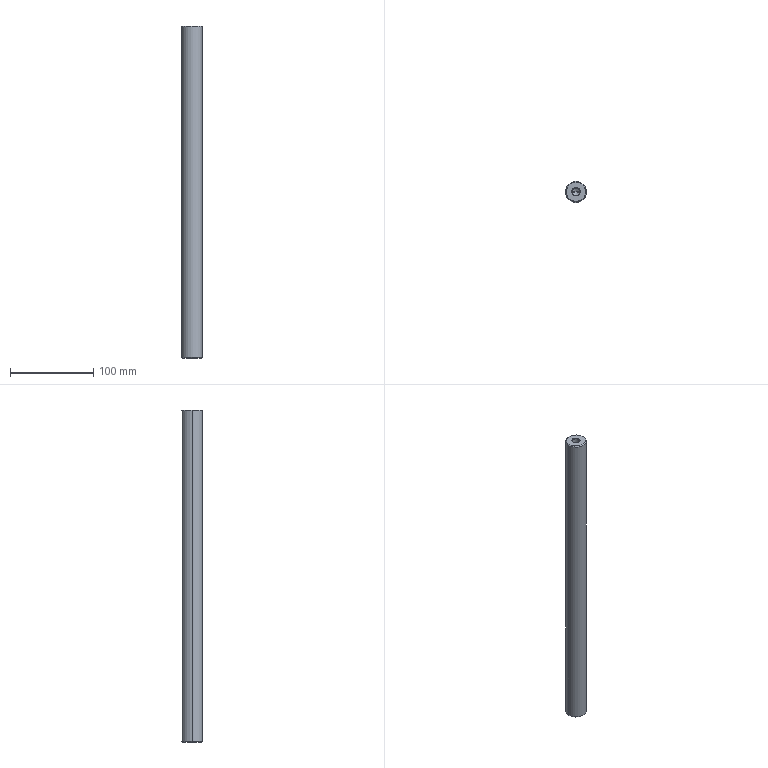Part | STEP file | 1 solid | 20 faces | box 25 x 25 x 400 mm | volume 193039 mm3 | cone 12 | cylinder 6 | plane 2 | commonest cylinder face diameters 8.5 x4 25 x2
STEP:
#1=CARTESIAN_POINT('',(0.,0.,0.));
#2=DIRECTION('',(0.,0.,1.));
#3=DIRECTION('',(1.,0.,0.));
#4=AXIS2_PLACEMENT_3D('',#1,#2,#3);
#5=CARTESIAN_POINT('',(-4.25,0.,-199.225));
#6=VERTEX_POINT('',#5);
#7=CARTESIAN_POINT('',(-5.025,0.,-200.));
#8=VERTEX_POINT('',#7);
#9=CARTESIAN_POINT('',(-5.025,0.,-200.));
#10=DIRECTION('',(-0.7071,0.,-0.7071));
#11=VECTOR('',#10,1.);
#12=LINE('',#9,#11);
#13=CARTESIAN_POINT('',(0.,0.,-200.));
#14=DIRECTION('',(0.,0.,-1.));
#15=DIRECTION('',(-1.,0.,0.));
#16=AXIS2_PLACEMENT_3D('',#13,#14,#15);
#17=CONICAL_SURFACE('',#16,5.025,0.7854);
#18=CARTESIAN_POINT('',(6.283,0.));
#19=DIRECTION('',(0.,1.));
#20=VECTOR('',#19,1.);
#21=LINE('',#18,#20);
#22=(GEOMETRIC_REPRESENTATION_CONTEXT(2)PARAMETRIC_REPRESENTATION_CONTEXT()REPRESENTATION_CONTEXT('',''));
#23=DEFINITIONAL_REPRESENTATION('',(#21),#22);
#24=PCURVE('',#17,#23);
#25=CARTESIAN_POINT('',(0.,0.,-200.));
#26=DIRECTION('',(0.,0.,-1.));
#27=DIRECTION('',(-1.,0.,0.));
#28=AXIS2_PLACEMENT_3D('',#25,#26,#27);
#29=CONICAL_SURFACE('',#28,5.025,0.7854);
#30=CARTESIAN_POINT('',(0.,0.));
#31=DIRECTION('',(0.,1.));
#32=VECTOR('',#31,1.);
#33=LINE('',#30,#32);
#34=(GEOMETRIC_REPRESENTATION_CONTEXT(2)PARAMETRIC_REPRESENTATION_CONTEXT()REPRESENTATION_CONTEXT('',''));
#35=DEFINITIONAL_REPRESENTATION('',(#33),#34);
#36=PCURVE('',#29,#35);
#37=SURFACE_CURVE('',#12,(#24,#36),.PCURVE_S1.);
#38=EDGE_CURVE('',#6,#8,#37,.T.);
#39=ORIENTED_EDGE('',*,*,#38,.T.);
#40=CARTESIAN_POINT('',(5.025,0.,-200.));
#41=VERTEX_POINT('',#40);
#42=CARTESIAN_POINT('',(0.,0.,-200.));
#43=DIRECTION('',(0.,0.,-1.));
#44=DIRECTION('',(-1.,0.,0.));
#45=AXIS2_PLACEMENT_3D('',#42,#43,#44);
#46=CIRCLE('',#45,5.025);
#47=CARTESIAN_POINT('',(0.,0.));
#48=DIRECTION('',(1.,0.));
#49=VECTOR('',#48,1.);
#50=LINE('',#47,#49);
#51=(GEOMETRIC_REPRESENTATION_CONTEXT(2)PARAMETRIC_REPRESENTATION_CONTEXT()REPRESENTATION_CONTEXT('',''));
#52=DEFINITIONAL_REPRESENTATION('',(#50),#51);
#53=PCURVE('',#17,#52);
#54=CARTESIAN_POINT('',(0.,0.,-200.));
#55=DIRECTION('',(0.,0.,1.));
#56=DIRECTION('',(1.,0.,0.));
#57=AXIS2_PLACEMENT_3D('',#54,#55,#56);
#58=PLANE('',#57);
#59=CARTESIAN_POINT('',(-5.025,0.));
#60=CARTESIAN_POINT('',(-5.025,8.704));
#61=CARTESIAN_POINT('',(2.513,4.352));
#62=CARTESIAN_POINT('',(10.05,0.));
#63=CARTESIAN_POINT('',(2.513,-4.352));
#64=CARTESIAN_POINT('',(-5.025,-8.704));
#65=CARTESIAN_POINT('',(-5.025,0.));
#66=(BOUNDED_CURVE()B_SPLINE_CURVE(2,(#59,#60,#61,#62,#63,#64,#65),.UNSPECIFIED.,.T.,.F.)B_SPLINE_CURVE_WITH_KNOTS((1,2,2,2,2,1),(-2.094,0.,2.094,4.189,6.283,8.378),.UNSPECIFIED.)CURVE()GEOMETRIC_REPRESENTATION_ITEM()RATIONAL_B_SPLINE_CURVE((1.,0.5,1.,0.5,1.,0.5,1.))REPRESENTATION_ITEM(''));
#67=(GEOMETRIC_REPRESENTATION_CONTEXT(2)PARAMETRIC_REPRESENTATION_CONTEXT()REPRESENTATION_CONTEXT('',''));
#68=DEFINITIONAL_REPRESENTATION('',(#66),#67);
#69=PCURVE('',#58,#68);
#70=SURFACE_CURVE('',#46,(#53,#69),.PCURVE_S1.);
#71=EDGE_CURVE('',#41,#8,#70,.T.);
#72=ORIENTED_EDGE('',*,*,#71,.F.);
#73=CARTESIAN_POINT('',(4.25,0.,-199.225));
#74=VERTEX_POINT('',#73);
#75=CARTESIAN_POINT('',(5.025,0.,-200.));
#76=DIRECTION('',(0.7071,0.,-0.7071));
#77=VECTOR('',#76,1.);
#78=LINE('',#75,#77);
#79=CARTESIAN_POINT('',(3.142,0.));
#80=DIRECTION('',(0.,1.));
#81=VECTOR('',#80,1.);
#82=LINE('',#79,#81);
#83=(GEOMETRIC_REPRESENTATION_CONTEXT(2)PARAMETRIC_REPRESENTATION_CONTEXT()REPRESENTATION_CONTEXT('',''));
#84=DEFINITIONAL_REPRESENTATION('',(#82),#83);
#85=PCURVE('',#17,#84);
#86=CARTESIAN_POINT('',(3.142,0.));
#87=DIRECTION('',(0.,1.));
#88=VECTOR('',#87,1.);
#89=LINE('',#86,#88);
#90=(GEOMETRIC_REPRESENTATION_CONTEXT(2)PARAMETRIC_REPRESENTATION_CONTEXT()REPRESENTATION_CONTEXT('',''));
#91=DEFINITIONAL_REPRESENTATION('',(#89),#90);
#92=PCURVE('',#29,#91);
#93=SURFACE_CURVE('',#78,(#85,#92),.PCURVE_S1.);
#94=EDGE_CURVE('',#74,#41,#93,.T.);
#95=ORIENTED_EDGE('',*,*,#94,.F.);
#96=CARTESIAN_POINT('',(0.,0.,-199.225));
#97=DIRECTION('',(0.,0.,-1.));
#98=DIRECTION('',(-1.,0.,0.));
#99=AXIS2_PLACEMENT_3D('',#96,#97,#98);
#100=CIRCLE('',#99,4.25);
#101=CARTESIAN_POINT('',(0.,-0.775));
#102=DIRECTION('',(1.,0.));
#103=VECTOR('',#102,1.);
#104=LINE('',#101,#103);
#105=(GEOMETRIC_REPRESENTATION_CONTEXT(2)PARAMETRIC_REPRESENTATION_CONTEXT()REPRESENTATION_CONTEXT('',''));
#106=DEFINITIONAL_REPRESENTATION('',(#104),#105);
#107=PCURVE('',#17,#106);
#108=CARTESIAN_POINT('',(0.,0.,-200.));
#109=DIRECTION('',(0.,0.,-1.));
#110=DIRECTION('',(-1.,0.,0.));
#111=AXIS2_PLACEMENT_3D('',#108,#109,#110);
#112=CYLINDRICAL_SURFACE('',#111,4.25);
#113=CARTESIAN_POINT('',(0.,-0.775));
#114=DIRECTION('',(1.,0.));
#115=VECTOR('',#114,1.);
#116=LINE('',#113,#115);
#117=(GEOMETRIC_REPRESENTATION_CONTEXT(2)PARAMETRIC_REPRESENTATION_CONTEXT()REPRESENTATION_CONTEXT('',''));
#118=DEFINITIONAL_REPRESENTATION('',(#116),#117);
#119=PCURVE('',#112,#118);
#120=SURFACE_CURVE('',#100,(#107,#119),.PCURVE_S1.);
#121=EDGE_CURVE('',#74,#6,#120,.T.);
#122=ORIENTED_EDGE('',*,*,#121,.T.);
#123=EDGE_LOOP('',(#39,#72,#95,#122));
#124=FACE_BOUND('',#123,.F.);
#125=ADVANCED_FACE('',(#124),#17,.F.);
#126=CARTESIAN_POINT('',(-4.25,0.,-172.5));
#127=VERTEX_POINT('',#126);
#128=CARTESIAN_POINT('',(-4.25,0.,-200.));
#129=DIRECTION('',(0.,0.,-1.));
#130=VECTOR('',#129,1.);
#131=LINE('',#128,#130);
#132=CARTESIAN_POINT('',(6.283,0.));
#133=DIRECTION('',(0.,1.));
#134=VECTOR('',#133,1.);
#135=LINE('',#132,#134);
#136=(GEOMETRIC_REPRESENTATION_CONTEXT(2)PARAMETRIC_REPRESENTATION_CONTEXT()REPRESENTATION_CONTEXT('',''));
#137=DEFINITIONAL_REPRESENTATION('',(#135),#136);
#138=PCURVE('',#112,#137);
#139=CARTESIAN_POINT('',(0.,0.,-200.));
#140=DIRECTION('',(0.,0.,-1.));
#141=DIRECTION('',(-1.,0.,0.));
#142=AXIS2_PLACEMENT_3D('',#139,#140,#141);
#143=CYLINDRICAL_SURFACE('',#142,4.25);
#144=CARTESIAN_POINT('',(0.,0.));
#145=DIRECTION('',(0.,1.));
#146=VECTOR('',#145,1.);
#147=LINE('',#144,#146);
#148=(GEOMETRIC_REPRESENTATION_CONTEXT(2)PARAMETRIC_REPRESENTATION_CONTEXT()REPRESENTATION_CONTEXT('',''));
#149=DEFINITIONAL_REPRESENTATION('',(#147),#148);
#150=PCURVE('',#143,#149);
#151=SURFACE_CURVE('',#131,(#138,#150),.PCURVE_S1.);
#152=EDGE_CURVE('',#127,#6,#151,.T.);
#153=ORIENTED_EDGE('',*,*,#152,.T.);
#154=ORIENTED_EDGE('',*,*,#121,.F.);
#155=CARTESIAN_POINT('',(4.25,0.,-172.5));
#156=VERTEX_POINT('',#155);
#157=CARTESIAN_POINT('',(4.25,0.,-200.));
#158=DIRECTION('',(0.,0.,-1.));
#159=VECTOR('',#158,1.);
#160=LINE('',#157,#159);
#161=CARTESIAN_POINT('',(3.142,0.));
#162=DIRECTION('',(0.,1.));
#163=VECTOR('',#162,1.);
#164=LINE('',#161,#163);
#165=(GEOMETRIC_REPRESENTATION_CONTEXT(2)PARAMETRIC_REPRESENTATION_CONTEXT()REPRESENTATION_CONTEXT('',''));
#166=DEFINITIONAL_REPRESENTATION('',(#164),#165);
#167=PCURVE('',#112,#166);
#168=CARTESIAN_POINT('',(3.142,0.));
#169=DIRECTION('',(0.,1.));
#170=VECTOR('',#169,1.);
#171=LINE('',#168,#170);
#172=(GEOMETRIC_REPRESENTATION_CONTEXT(2)PARAMETRIC_REPRESENTATION_CONTEXT()REPRESENTATION_CONTEXT('',''));
#173=DEFINITIONAL_REPRESENTATION('',(#171),#172);
#174=PCURVE('',#143,#173);
#175=SURFACE_CURVE('',#160,(#167,#174),.PCURVE_S1.);
#176=EDGE_CURVE('',#156,#74,#175,.T.);
#177=ORIENTED_EDGE('',*,*,#176,.F.);
#178=CARTESIAN_POINT('',(0.,0.,-172.5));
#179=DIRECTION('',(0.,0.,-1.));
#180=DIRECTION('',(-1.,0.,0.));
#181=AXIS2_PLACEMENT_3D('',#178,#179,#180);
#182=CIRCLE('',#181,4.25);
#183=CARTESIAN_POINT('',(0.,-27.5));
#184=DIRECTION('',(1.,0.));
#185=VECTOR('',#184,1.);
#186=LINE('',#183,#185);
#187=(GEOMETRIC_REPRESENTATION_CONTEXT(2)PARAMETRIC_REPRESENTATION_CONTEXT()REPRESENTATION_CONTEXT('',''));
#188=DEFINITIONAL_REPRESENTATION('',(#186),#187);
#189=PCURVE('',#112,#188);
#190=CARTESIAN_POINT('',(0.,0.,-172.5));
#191=DIRECTION('',(0.,0.,-1.));
#192=DIRECTION('',(-1.,0.,0.));
#193=AXIS2_PLACEMENT_3D('',#190,#191,#192);
#194=CONICAL_SURFACE('',#193,4.25,1.03);
#195=CARTESIAN_POINT('',(0.,0.));
#196=DIRECTION('',(1.,0.));
#197=VECTOR('',#196,1.);
#198=LINE('',#195,#197);
#199=(GEOMETRIC_REPRESENTATION_CONTEXT(2)PARAMETRIC_REPRESENTATION_CONTEXT()REPRESENTATION_CONTEXT('',''));
#200=DEFINITIONAL_REPRESENTATION('',(#198),#199);
#201=PCURVE('',#194,#200);
#202=SURFACE_CURVE('',#182,(#189,#201),.PCURVE_S1.);
#203=EDGE_CURVE('',#156,#127,#202,.T.);
#204=ORIENTED_EDGE('',*,*,#203,.T.);
#205=EDGE_LOOP('',(#153,#154,#177,#204));
#206=FACE_BOUND('',#205,.F.);
#207=ADVANCED_FACE('',(#206),#112,.F.);
#208=ORIENTED_EDGE('',*,*,#203,.F.);
#209=CARTESIAN_POINT('',(0.,0.,-169.946));
#210=VERTEX_POINT('',#209);
#211=CARTESIAN_POINT('',(4.25,0.,-172.5));
#212=DIRECTION('',(0.8572,0.,-0.515));
#213=VECTOR('',#212,1.);
#214=LINE('',#211,#213);
#215=CARTESIAN_POINT('',(3.142,0.));
#216=DIRECTION('',(0.,1.));
#217=VECTOR('',#216,1.);
#218=LINE('',#215,#217);
#219=(GEOMETRIC_REPRESENTATION_CONTEXT(2)PARAMETRIC_REPRESENTATION_CONTEXT()REPRESENTATION_CONTEXT('',''));
#220=DEFINITIONAL_REPRESENTATION('',(#218),#219);
#221=PCURVE('',#194,#220);
#222=CARTESIAN_POINT('',(0.,0.,-172.5));
#223=DIRECTION('',(0.,0.,-1.));
#224=DIRECTION('',(-1.,0.,0.));
#225=AXIS2_PLACEMENT_3D('',#222,#223,#224);
#226=CONICAL_SURFACE('',#225,4.25,1.03);
#227=CARTESIAN_POINT('',(3.142,0.));
#228=DIRECTION('',(0.,1.));
#229=VECTOR('',#228,1.);
#230=LINE('',#227,#229);
#231=(GEOMETRIC_REPRESENTATION_CONTEXT(2)PARAMETRIC_REPRESENTATION_CONTEXT()REPRESENTATION_CONTEXT('',''));
#232=DEFINITIONAL_REPRESENTATION('',(#230),#231);
#233=PCURVE('',#226,#232);
#234=SURFACE_CURVE('',#214,(#221,#233),.PCURVE_S1.);
#235=EDGE_CURVE('',#210,#156,#234,.T.);
#236=ORIENTED_EDGE('',*,*,#235,.F.);
#237=CARTESIAN_POINT('',(-4.25,0.,-172.5));
#238=DIRECTION('',(-0.8572,0.,-0.515));
#239=VECTOR('',#238,1.);
#240=LINE('',#237,#239);
#241=CARTESIAN_POINT('',(6.283,0.));
#242=DIRECTION('',(0.,1.));
#243=VECTOR('',#242,1.);
#244=LINE('',#241,#243);
#245=(GEOMETRIC_REPRESENTATION_CONTEXT(2)PARAMETRIC_REPRESENTATION_CONTEXT()REPRESENTATION_CONTEXT('',''));
#246=DEFINITIONAL_REPRESENTATION('',(#244),#245);
#247=PCURVE('',#194,#246);
#248=CARTESIAN_POINT('',(0.,0.));
#249=DIRECTION('',(0.,1.));
#250=VECTOR('',#249,1.);
#251=LINE('',#248,#250);
#252=(GEOMETRIC_REPRESENTATION_CONTEXT(2)PARAMETRIC_REPRESENTATION_CONTEXT()REPRESENTATION_CONTEXT('',''));
#253=DEFINITIONAL_REPRESENTATION('',(#251),#252);
#254=PCURVE('',#226,#253);
#255=SURFACE_CURVE('',#240,(#247,#254),.PCURVE_S1.);
#256=EDGE_CURVE('',#210,#127,#255,.T.);
#257=ORIENTED_EDGE('',*,*,#256,.T.);
#258=EDGE_LOOP('',(#208,#236,#257));
#259=FACE_BOUND('',#258,.F.);
#260=ADVANCED_FACE('',(#259),#194,.F.);
#261=CARTESIAN_POINT('',(4.25,0.,199.225));
#262=VERTEX_POINT('',#261);
#263=CARTESIAN_POINT('',(5.025,0.,200.));
#264=VERTEX_POINT('',#263);
#265=CARTESIAN_POINT('',(5.025,0.,200.));
#266=DIRECTION('',(0.7071,0.,0.7071));
#267=VECTOR('',#266,1.);
#268=LINE('',#265,#267);
#269=CARTESIAN_POINT('',(0.,0.,200.));
#270=DIRECTION('',(0.,0.,1.));
#271=DIRECTION('',(1.,0.,0.));
#272=AXIS2_PLACEMENT_3D('',#269,#270,#271);
#273=CONICAL_SURFACE('',#272,5.025,0.7854);
#274=CARTESIAN_POINT('',(6.283,0.));
#275=DIRECTION('',(0.,1.));
#276=VECTOR('',#275,1.);
#277=LINE('',#274,#276);
#278=(GEOMETRIC_REPRESENTATION_CONTEXT(2)PARAMETRIC_REPRESENTATION_CONTEXT()REPRESENTATION_CONTEXT('',''));
#279=DEFINITIONAL_REPRESENTATION('',(#277),#278);
#280=PCURVE('',#273,#279);
#281=CARTESIAN_POINT('',(0.,0.,200.));
#282=DIRECTION('',(0.,0.,1.));
#283=DIRECTION('',(1.,0.,0.));
#284=AXIS2_PLACEMENT_3D('',#281,#282,#283);
#285=CONICAL_SURFACE('',#284,5.025,0.7854);
#286=CARTESIAN_POINT('',(0.,0.));
#287=DIRECTION('',(0.,1.));
#288=VECTOR('',#287,1.);
#289=LINE('',#286,#288);
#290=(GEOMETRIC_REPRESENTATION_CONTEXT(2)PARAMETRIC_REPRESENTATION_CONTEXT()REPRESENTATION_CONTEXT('',''));
#291=DEFINITIONAL_REPRESENTATION('',(#289),#290);
#292=PCURVE('',#285,#291);
#293=SURFACE_CURVE('',#268,(#280,#292),.PCURVE_S1.);
#294=EDGE_CURVE('',#262,#264,#293,.T.);
#295=ORIENTED_EDGE('',*,*,#294,.T.);
#296=CARTESIAN_POINT('',(-5.025,0.,200.));
#297=VERTEX_POINT('',#296);
#298=CARTESIAN_POINT('',(0.,0.,200.));
#299=DIRECTION('',(0.,0.,1.));
#300=DIRECTION('',(1.,0.,0.));
#301=AXIS2_PLACEMENT_3D('',#298,#299,#300);
#302=CIRCLE('',#301,5.025);
#303=CARTESIAN_POINT('',(0.,0.));
#304=DIRECTION('',(1.,0.));
#305=VECTOR('',#304,1.);
#306=LINE('',#303,#305);
#307=(GEOMETRIC_REPRESENTATION_CONTEXT(2)PARAMETRIC_REPRESENTATION_CONTEXT()REPRESENTATION_CONTEXT('',''));
#308=DEFINITIONAL_REPRESENTATION('',(#306),#307);
#309=PCURVE('',#273,#308);
#310=CARTESIAN_POINT('',(0.,0.,200.));
#311=DIRECTION('',(0.,0.,1.));
#312=DIRECTION('',(1.,0.,0.));
#313=AXIS2_PLACEMENT_3D('',#310,#311,#312);
#314=PLANE('',#313);
#315=CARTESIAN_POINT('',(0.,0.));
#316=DIRECTION('',(1.,0.));
#317=AXIS2_PLACEMENT_2D('',#315,#316);
#318=CIRCLE('',#317,5.025);
#319=(GEOMETRIC_REPRESENTATION_CONTEXT(2)PARAMETRIC_REPRESENTATION_CONTEXT()REPRESENTATION_CONTEXT('',''));
#320=DEFINITIONAL_REPRESENTATION('',(#318),#319);
#321=PCURVE('',#314,#320);
#322=SURFACE_CURVE('',#302,(#309,#321),.PCURVE_S1.);
#323=EDGE_CURVE('',#297,#264,#322,.T.);
#324=ORIENTED_EDGE('',*,*,#323,.F.);
#325=CARTESIAN_POINT('',(-4.25,0.,199.225));
#326=VERTEX_POINT('',#325);
#327=CARTESIAN_POINT('',(-5.025,0.,200.));
#328=DIRECTION('',(-0.7071,0.,0.7071));
#329=VECTOR('',#328,1.);
#330=LINE('',#327,#329);
#331=CARTESIAN_POINT('',(3.142,0.));
#332=DIRECTION('',(0.,1.));
#333=VECTOR('',#332,1.);
#334=LINE('',#331,#333);
#335=(GEOMETRIC_REPRESENTATION_CONTEXT(2)PARAMETRIC_REPRESENTATION_CONTEXT()REPRESENTATION_CONTEXT('',''));
#336=DEFINITIONAL_REPRESENTATION('',(#334),#335);
#337=PCURVE('',#273,#336);
#338=CARTESIAN_POINT('',(3.142,0.));
#339=DIRECTION('',(0.,1.));
#340=VECTOR('',#339,1.);
#341=LINE('',#338,#340);
#342=(GEOMETRIC_REPRESENTATION_CONTEXT(2)PARAMETRIC_REPRESENTATION_CONTEXT()REPRESENTATION_CONTEXT('',''));
#343=DEFINITIONAL_REPRESENTATION('',(#341),#342);
#344=PCURVE('',#285,#343);
#345=SURFACE_CURVE('',#330,(#337,#344),.PCURVE_S1.);
#346=EDGE_CURVE('',#326,#297,#345,.T.);
#347=ORIENTED_EDGE('',*,*,#346,.F.);
#348=CARTESIAN_POINT('',(0.,0.,199.225));
#349=DIRECTION('',(0.,0.,1.));
#350=DIRECTION('',(1.,0.,0.));
#351=AXIS2_PLACEMENT_3D('',#348,#349,#350);
#352=CIRCLE('',#351,4.25);
#353=CARTESIAN_POINT('',(0.,-0.775));
#354=DIRECTION('',(1.,0.));
#355=VECTOR('',#354,1.);
#356=LINE('',#353,#355);
#357=(GEOMETRIC_REPRESENTATION_CONTEXT(2)PARAMETRIC_REPRESENTATION_CONTEXT()REPRESENTATION_CONTEXT('',''));
#358=DEFINITIONAL_REPRESENTATION('',(#356),#357);
#359=PCURVE('',#273,#358);
#360=CARTESIAN_POINT('',(0.,0.,200.));
#361=DIRECTION('',(0.,0.,1.));
#362=DIRECTION('',(1.,0.,0.));
#363=AXIS2_PLACEMENT_3D('',#360,#361,#362);
#364=CYLINDRICAL_SURFACE('',#363,4.25);
#365=CARTESIAN_POINT('',(0.,-0.775));
#366=DIRECTION('',(1.,0.));
#367=VECTOR('',#366,1.);
#368=LINE('',#365,#367);
#369=(GEOMETRIC_REPRESENTATION_CONTEXT(2)PARAMETRIC_REPRESENTATION_CONTEXT()REPRESENTATION_CONTEXT('',''));
#370=DEFINITIONAL_REPRESENTATION('',(#368),#369);
#371=PCURVE('',#364,#370);
#372=SURFACE_CURVE('',#352,(#359,#371),.PCURVE_S1.);
#373=EDGE_CURVE('',#326,#262,#372,.T.);
#374=ORIENTED_EDGE('',*,*,#373,.T.);
#375=EDGE_LOOP('',(#295,#324,#347,#374));
#376=FACE_BOUND('',#375,.F.);
#377=ADVANCED_FACE('',(#376),#273,.F.);
#378=CARTESIAN_POINT('',(4.25,0.,172.5));
#379=VERTEX_POINT('',#378);
#380=CARTESIAN_POINT('',(4.25,0.,200.));
#381=DIRECTION('',(0.,0.,1.));
#382=VECTOR('',#381,1.);
#383=LINE('',#380,#382);
#384=CARTESIAN_POINT('',(6.283,0.));
#385=DIRECTION('',(0.,1.));
#386=VECTOR('',#385,1.);
#387=LINE('',#384,#386);
#388=(GEOMETRIC_REPRESENTATION_CONTEXT(2)PARAMETRIC_REPRESENTATION_CONTEXT()REPRESENTATION_CONTEXT('',''));
#389=DEFINITIONAL_REPRESENTATION('',(#387),#388);
#390=PCURVE('',#364,#389);
#391=CARTESIAN_POINT('',(0.,0.,200.));
#392=DIRECTION('',(0.,0.,1.));
#393=DIRECTION('',(1.,0.,0.));
#394=AXIS2_PLACEMENT_3D('',#391,#392,#393);
#395=CYLINDRICAL_SURFACE('',#394,4.25);
#396=CARTESIAN_POINT('',(0.,0.));
#397=DIRECTION('',(0.,1.));
#398=VECTOR('',#397,1.);
#399=LINE('',#396,#398);
#400=(GEOMETRIC_REPRESENTATION_CONTEXT(2)PARAMETRIC_REPRESENTATION_CONTEXT()REPRESENTATION_CONTEXT('',''));
#401=DEFINITIONAL_REPRESENTATION('',(#399),#400);
#402=PCURVE('',#395,#401);
#403=SURFACE_CURVE('',#383,(#390,#402),.PCURVE_S1.);
#404=EDGE_CURVE('',#379,#262,#403,.T.);
#405=ORIENTED_EDGE('',*,*,#404,.T.);
#406=ORIENTED_EDGE('',*,*,#373,.F.);
#407=CARTESIAN_POINT('',(-4.25,0.,172.5));
#408=VERTEX_POINT('',#407);
#409=CARTESIAN_POINT('',(-4.25,0.,200.));
#410=DIRECTION('',(0.,0.,1.));
#411=VECTOR('',#410,1.);
#412=LINE('',#409,#411);
#413=CARTESIAN_POINT('',(3.142,0.));
#414=DIRECTION('',(0.,1.));
#415=VECTOR('',#414,1.);
#416=LINE('',#413,#415);
#417=(GEOMETRIC_REPRESENTATION_CONTEXT(2)PARAMETRIC_REPRESENTATION_CONTEXT()REPRESENTATION_CONTEXT('',''));
#418=DEFINITIONAL_REPRESENTATION('',(#416),#417);
#419=PCURVE('',#364,#418);
#420=CARTESIAN_POINT('',(3.142,0.));
#421=DIRECTION('',(0.,1.));
#422=VECTOR('',#421,1.);
#423=LINE('',#420,#422);
#424=(GEOMETRIC_REPRESENTATION_CONTEXT(2)PARAMETRIC_REPRESENTATION_CONTEXT()REPRESENTATION_CONTEXT('',''));
#425=DEFINITIONAL_REPRESENTATION('',(#423),#424);
#426=PCURVE('',#395,#425);
#427=SURFACE_CURVE('',#412,(#419,#426),.PCURVE_S1.);
#428=EDGE_CURVE('',#408,#326,#427,.T.);
#429=ORIENTED_EDGE('',*,*,#428,.F.);
#430=CARTESIAN_POINT('',(0.,0.,172.5));
#431=DIRECTION('',(0.,0.,1.));
#432=DIRECTION('',(1.,0.,0.));
#433=AXIS2_PLACEMENT_3D('',#430,#431,#432);
#434=CIRCLE('',#433,4.25);
#435=CARTESIAN_POINT('',(0.,-27.5));
#436=DIRECTION('',(1.,0.));
#437=VECTOR('',#436,1.);
#438=LINE('',#435,#437);
#439=(GEOMETRIC_REPRESENTATION_CONTEXT(2)PARAMETRIC_REPRESENTATION_CONTEXT()REPRESENTATION_CONTEXT('',''));
#440=DEFINITIONAL_REPRESENTATION('',(#438),#439);
#441=PCURVE('',#364,#440);
#442=CARTESIAN_POINT('',(0.,0.,172.5));
#443=DIRECTION('',(0.,0.,1.));
#444=DIRECTION('',(1.,0.,0.));
#445=AXIS2_PLACEMENT_3D('',#442,#443,#444);
#446=CONICAL_SURFACE('',#445,4.25,1.03);
#447=CARTESIAN_POINT('',(0.,0.));
#448=DIRECTION('',(1.,0.));
#449=VECTOR('',#448,1.);
#450=LINE('',#447,#449);
#451=(GEOMETRIC_REPRESENTATION_CONTEXT(2)PARAMETRIC_REPRESENTATION_CONTEXT()REPRESENTATION_CONTEXT('',''));
#452=DEFINITIONAL_REPRESENTATION('',(#450),#451);
#453=PCURVE('',#446,#452);
#454=SURFACE_CURVE('',#434,(#441,#453),.PCURVE_S1.);
#455=EDGE_CURVE('',#408,#379,#454,.T.);
#456=ORIENTED_EDGE('',*,*,#455,.T.);
#457=EDGE_LOOP('',(#405,#406,#429,#456));
#458=FACE_BOUND('',#457,.F.);
#459=ADVANCED_FACE('',(#458),#364,.F.);
#460=ORIENTED_EDGE('',*,*,#455,.F.);
#461=CARTESIAN_POINT('',(0.,0.,169.946));
#462=VERTEX_POINT('',#461);
#463=CARTESIAN_POINT('',(-4.25,0.,172.5));
#464=DIRECTION('',(-0.8572,0.,0.515));
#465=VECTOR('',#464,1.);
#466=LINE('',#463,#465);
#467=CARTESIAN_POINT('',(3.142,0.));
#468=DIRECTION('',(0.,1.));
#469=VECTOR('',#468,1.);
#470=LINE('',#467,#469);
#471=(GEOMETRIC_REPRESENTATION_CONTEXT(2)PARAMETRIC_REPRESENTATION_CONTEXT()REPRESENTATION_CONTEXT('',''));
#472=DEFINITIONAL_REPRESENTATION('',(#470),#471);
#473=PCURVE('',#446,#472);
#474=CARTESIAN_POINT('',(0.,0.,172.5));
#475=DIRECTION('',(0.,0.,1.));
#476=DIRECTION('',(1.,0.,0.));
#477=AXIS2_PLACEMENT_3D('',#474,#475,#476);
#478=CONICAL_SURFACE('',#477,4.25,1.03);
#479=CARTESIAN_POINT('',(3.142,0.));
#480=DIRECTION('',(0.,1.));
#481=VECTOR('',#480,1.);
#482=LINE('',#479,#481);
#483=(GEOMETRIC_REPRESENTATION_CONTEXT(2)PARAMETRIC_REPRESENTATION_CONTEXT()REPRESENTATION_CONTEXT('',''));
#484=DEFINITIONAL_REPRESENTATION('',(#482),#483);
#485=PCURVE('',#478,#484);
#486=SURFACE_CURVE('',#466,(#473,#485),.PCURVE_S1.);
#487=EDGE_CURVE('',#462,#408,#486,.T.);
#488=ORIENTED_EDGE('',*,*,#487,.F.);
#489=CARTESIAN_POINT('',(4.25,0.,172.5));
#490=DIRECTION('',(0.8572,0.,0.515));
#491=VECTOR('',#490,1.);
#492=LINE('',#489,#491);
#493=CARTESIAN_POINT('',(6.283,0.));
#494=DIRECTION('',(0.,1.));
#495=VECTOR('',#494,1.);
#496=LINE('',#493,#495);
#497=(GEOMETRIC_REPRESENTATION_CONTEXT(2)PARAMETRIC_REPRESENTATION_CONTEXT()REPRESENTATION_CONTEXT('',''));
#498=DEFINITIONAL_REPRESENTATION('',(#496),#497);
#499=PCURVE('',#446,#498);
#500=CARTESIAN_POINT('',(0.,0.));
#501=DIRECTION('',(0.,1.));
#502=VECTOR('',#501,1.);
#503=LINE('',#500,#502);
#504=(GEOMETRIC_REPRESENTATION_CONTEXT(2)PARAMETRIC_REPRESENTATION_CONTEXT()REPRESENTATION_CONTEXT('',''));
#505=DEFINITIONAL_REPRESENTATION('',(#503),#504);
#506=PCURVE('',#478,#505);
#507=SURFACE_CURVE('',#492,(#499,#506),.PCURVE_S1.);
#508=EDGE_CURVE('',#462,#379,#507,.T.);
#509=ORIENTED_EDGE('',*,*,#508,.T.);
#510=EDGE_LOOP('',(#460,#488,#509));
#511=FACE_BOUND('',#510,.F.);
#512=ADVANCED_FACE('',(#511),#446,.F.);
#513=CARTESIAN_POINT('',(11.5,0.,200.));
#514=VERTEX_POINT('',#513);
#515=CARTESIAN_POINT('',(-11.5,0.,200.));
#516=VERTEX_POINT('',#515);
#517=CARTESIAN_POINT('',(0.,0.,200.));
#518=DIRECTION('',(0.,0.,1.));
#519=DIRECTION('',(1.,0.,0.));
#520=AXIS2_PLACEMENT_3D('',#517,#518,#519);
#521=CIRCLE('',#520,11.5);
#522=CARTESIAN_POINT('',(0.,0.,200.));
#523=DIRECTION('',(0.,0.,-1.));
#524=DIRECTION('',(-1.,0.,0.));
#525=AXIS2_PLACEMENT_3D('',#522,#523,#524);
#526=CONICAL_SURFACE('',#525,11.5,0.7854);
#527=CARTESIAN_POINT('',(3.142,0.));
#528=DIRECTION('',(-1.,0.));
#529=VECTOR('',#528,1.);
#530=LINE('',#527,#529);
#531=(GEOMETRIC_REPRESENTATION_CONTEXT(2)PARAMETRIC_REPRESENTATION_CONTEXT()REPRESENTATION_CONTEXT('',''));
#532=DEFINITIONAL_REPRESENTATION('',(#530),#531);
#533=PCURVE('',#526,#532);
#534=CARTESIAN_POINT('',(0.,0.));
#535=DIRECTION('',(1.,0.));
#536=AXIS2_PLACEMENT_2D('',#534,#535);
#537=CIRCLE('',#536,11.5);
#538=(GEOMETRIC_REPRESENTATION_CONTEXT(2)PARAMETRIC_REPRESENTATION_CONTEXT()REPRESENTATION_CONTEXT('',''));
#539=DEFINITIONAL_REPRESENTATION('',(#537),#538);
#540=PCURVE('',#314,#539);
#541=SURFACE_CURVE('',#521,(#533,#540),.PCURVE_S1.);
#542=EDGE_CURVE('',#514,#516,#541,.T.);
#543=ORIENTED_EDGE('',*,*,#542,.F.);
#544=CARTESIAN_POINT('',(12.5,0.,199.));
#545=VERTEX_POINT('',#544);
#546=CARTESIAN_POINT('',(11.5,0.,200.));
#547=DIRECTION('',(0.7071,0.,-0.7071));
#548=VECTOR('',#547,1.);
#549=LINE('',#546,#548);
#550=CARTESIAN_POINT('',(3.142,0.));
#551=DIRECTION('',(0.,1.));
#552=VECTOR('',#551,1.);
#553=LINE('',#550,#552);
#554=(GEOMETRIC_REPRESENTATION_CONTEXT(2)PARAMETRIC_REPRESENTATION_CONTEXT()REPRESENTATION_CONTEXT('',''));
#555=DEFINITIONAL_REPRESENTATION('',(#553),#554);
#556=PCURVE('',#526,#555);
#557=CARTESIAN_POINT('',(0.,0.,200.));
#558=DIRECTION('',(0.,0.,-1.));
#559=DIRECTION('',(-1.,0.,0.));
#560=AXIS2_PLACEMENT_3D('',#557,#558,#559);
#561=CONICAL_SURFACE('',#560,11.5,0.7854);
#562=CARTESIAN_POINT('',(3.142,0.));
#563=DIRECTION('',(0.,1.));
#564=VECTOR('',#563,1.);
#565=LINE('',#562,#564);
#566=(GEOMETRIC_REPRESENTATION_CONTEXT(2)PARAMETRIC_REPRESENTATION_CONTEXT()REPRESENTATION_CONTEXT('',''));
#567=DEFINITIONAL_REPRESENTATION('',(#565),#566);
#568=PCURVE('',#561,#567);
#569=SURFACE_CURVE('',#549,(#556,#568),.PCURVE_S1.);
#570=EDGE_CURVE('',#514,#545,#569,.T.);
#571=ORIENTED_EDGE('',*,*,#570,.T.);
#572=CARTESIAN_POINT('',(-12.5,0.,199.));
#573=VERTEX_POINT('',#572);
#574=CARTESIAN_POINT('',(0.,0.,199.));
#575=DIRECTION('',(0.,0.,-1.));
#576=DIRECTION('',(1.,0.,0.));
#577=AXIS2_PLACEMENT_3D('',#574,#575,#576);
#578=CIRCLE('',#577,12.5);
#579=CARTESIAN_POINT('',(-3.142,1.));
#580=DIRECTION('',(1.,0.));
#581=VECTOR('',#580,1.);
#582=LINE('',#579,#581);
#583=(GEOMETRIC_REPRESENTATION_CONTEXT(2)PARAMETRIC_REPRESENTATION_CONTEXT()REPRESENTATION_CONTEXT('',''));
#584=DEFINITIONAL_REPRESENTATION('',(#582),#583);
#585=PCURVE('',#526,#584);
#586=CARTESIAN_POINT('',(0.,0.,200.));
#587=DIRECTION('',(0.,0.,-1.));
#588=DIRECTION('',(-1.,0.,0.));
#589=AXIS2_PLACEMENT_3D('',#586,#587,#588);
#590=CYLINDRICAL_SURFACE('',#589,12.5);
#591=CARTESIAN_POINT('',(-3.142,1.));
#592=DIRECTION('',(1.,0.));
#593=VECTOR('',#592,1.);
#594=LINE('',#591,#593);
#595=(GEOMETRIC_REPRESENTATION_CONTEXT(2)PARAMETRIC_REPRESENTATION_CONTEXT()REPRESENTATION_CONTEXT('',''));
#596=DEFINITIONAL_REPRESENTATION('',(#594),#595);
#597=PCURVE('',#590,#596);
#598=SURFACE_CURVE('',#578,(#585,#597),.PCURVE_S1.);
#599=EDGE_CURVE('',#573,#545,#598,.T.);
#600=ORIENTED_EDGE('',*,*,#599,.F.);
#601=CARTESIAN_POINT('',(-11.5,0.,200.));
#602=DIRECTION('',(-0.7071,0.,-0.7071));
#603=VECTOR('',#602,1.);
#604=LINE('',#601,#603);
#605=CARTESIAN_POINT('',(0.,0.));
#606=DIRECTION('',(0.,1.));
#607=VECTOR('',#606,1.);
#608=LINE('',#605,#607);
#609=(GEOMETRIC_REPRESENTATION_CONTEXT(2)PARAMETRIC_REPRESENTATION_CONTEXT()REPRESENTATION_CONTEXT('',''));
#610=DEFINITIONAL_REPRESENTATION('',(#608),#609);
#611=PCURVE('',#526,#610);
#612=CARTESIAN_POINT('',(6.283,0.));
#613=DIRECTION('',(0.,1.));
#614=VECTOR('',#613,1.);
#615=LINE('',#612,#614);
#616=(GEOMETRIC_REPRESENTATION_CONTEXT(2)PARAMETRIC_REPRESENTATION_CONTEXT()REPRESENTATION_CONTEXT('',''));
#617=DEFINITIONAL_REPRESENTATION('',(#615),#616);
#618=PCURVE('',#561,#617);
#619=SURFACE_CURVE('',#604,(#611,#618),.PCURVE_S1.);
#620=EDGE_CURVE('',#516,#573,#619,.T.);
#621=ORIENTED_EDGE('',*,*,#620,.F.);
#622=EDGE_LOOP('',(#543,#571,#600,#621));
#623=FACE_BOUND('',#622,.T.);
#624=ADVANCED_FACE('',(#623),#526,.T.);
#625=CARTESIAN_POINT('',(-11.5,0.,-200.));
#626=VERTEX_POINT('',#625);
#627=CARTESIAN_POINT('',(11.5,0.,-200.));
#628=VERTEX_POINT('',#627);
#629=CARTESIAN_POINT('',(0.,0.,-200.));
#630=DIRECTION('',(0.,0.,-1.));
#631=DIRECTION('',(1.,0.,0.));
#632=AXIS2_PLACEMENT_3D('',#629,#630,#631);
#633=CIRCLE('',#632,11.5);
#634=CARTESIAN_POINT('',(0.,0.,-199.));
#635=DIRECTION('',(0.,0.,1.));
#636=DIRECTION('',(1.,0.,0.));
#637=AXIS2_PLACEMENT_3D('',#634,#635,#636);
#638=CONICAL_SURFACE('',#637,12.5,0.7854);
#639=CARTESIAN_POINT('',(6.283,-1.));
#640=DIRECTION('',(-1.,0.));
#641=VECTOR('',#640,1.);
#642=LINE('',#639,#641);
#643=(GEOMETRIC_REPRESENTATION_CONTEXT(2)PARAMETRIC_REPRESENTATION_CONTEXT()REPRESENTATION_CONTEXT('',''));
#644=DEFINITIONAL_REPRESENTATION('',(#642),#643);
#645=PCURVE('',#638,#644);
#646=CARTESIAN_POINT('',(11.5,0.));
#647=CARTESIAN_POINT('',(11.5,-19.919));
#648=CARTESIAN_POINT('',(-5.75,-9.959));
#649=CARTESIAN_POINT('',(-23.,0.));
#650=CARTESIAN_POINT('',(-5.75,9.959));
#651=CARTESIAN_POINT('',(11.5,19.919));
#652=CARTESIAN_POINT('',(11.5,0.));
#653=(BOUNDED_CURVE()B_SPLINE_CURVE(2,(#646,#647,#648,#649,#650,#651,#652),.UNSPECIFIED.,.T.,.F.)B_SPLINE_CURVE_WITH_KNOTS((1,2,2,2,2,1),(-2.094,0.,2.094,4.189,6.283,8.378),.UNSPECIFIED.)CURVE()GEOMETRIC_REPRESENTATION_ITEM()RATIONAL_B_SPLINE_CURVE((1.,0.5,1.,0.5,1.,0.5,1.))REPRESENTATION_ITEM(''));
#654=(GEOMETRIC_REPRESENTATION_CONTEXT(2)PARAMETRIC_REPRESENTATION_CONTEXT()REPRESENTATION_CONTEXT('',''));
#655=DEFINITIONAL_REPRESENTATION('',(#653),#654);
#656=PCURVE('',#58,#655);
#657=SURFACE_CURVE('',#633,(#645,#656),.PCURVE_S1.);
#658=EDGE_CURVE('',#626,#628,#657,.T.);
#659=ORIENTED_EDGE('',*,*,#658,.F.);
#660=CARTESIAN_POINT('',(-12.5,0.,-199.));
#661=VERTEX_POINT('',#660);
#662=CARTESIAN_POINT('',(-12.5,0.,-199.));
#663=DIRECTION('',(-0.7071,0.,0.7071));
#664=VECTOR('',#663,1.);
#665=LINE('',#662,#664);
#666=CARTESIAN_POINT('',(3.142,0.));
#667=DIRECTION('',(0.,1.));
#668=VECTOR('',#667,1.);
#669=LINE('',#666,#668);
#670=(GEOMETRIC_REPRESENTATION_CONTEXT(2)PARAMETRIC_REPRESENTATION_CONTEXT()REPRESENTATION_CONTEXT('',''));
#671=DEFINITIONAL_REPRESENTATION('',(#669),#670);
#672=PCURVE('',#638,#671);
#673=CARTESIAN_POINT('',(0.,0.,-199.));
#674=DIRECTION('',(0.,0.,1.));
#675=DIRECTION('',(1.,0.,0.));
#676=AXIS2_PLACEMENT_3D('',#673,#674,#675);
#677=CONICAL_SURFACE('',#676,12.5,0.7854);
#678=CARTESIAN_POINT('',(3.142,0.));
#679=DIRECTION('',(0.,1.));
#680=VECTOR('',#679,1.);
#681=LINE('',#678,#680);
#682=(GEOMETRIC_REPRESENTATION_CONTEXT(2)PARAMETRIC_REPRESENTATION_CONTEXT()REPRESENTATION_CONTEXT('',''));
#683=DEFINITIONAL_REPRESENTATION('',(#681),#682);
#684=PCURVE('',#677,#683);
#685=SURFACE_CURVE('',#665,(#672,#684),.PCURVE_S1.);
#686=EDGE_CURVE('',#626,#661,#685,.T.);
#687=ORIENTED_EDGE('',*,*,#686,.T.);
#688=CARTESIAN_POINT('',(12.5,0.,-199.));
#689=VERTEX_POINT('',#688);
#690=CARTESIAN_POINT('',(0.,0.,-199.));
#691=DIRECTION('',(0.,0.,1.));
#692=DIRECTION('',(1.,0.,0.));
#693=AXIS2_PLACEMENT_3D('',#690,#691,#692);
#694=CIRCLE('',#693,12.5);
#695=CARTESIAN_POINT('',(0.,0.));
#696=DIRECTION('',(1.,0.));
#697=VECTOR('',#696,1.);
#698=LINE('',#695,#697);
#699=(GEOMETRIC_REPRESENTATION_CONTEXT(2)PARAMETRIC_REPRESENTATION_CONTEXT()REPRESENTATION_CONTEXT('',''));
#700=DEFINITIONAL_REPRESENTATION('',(#698),#699);
#701=PCURVE('',#638,#700);
#702=CARTESIAN_POINT('',(3.142,399.));
#703=DIRECTION('',(-1.,0.));
#704=VECTOR('',#703,1.);
#705=LINE('',#702,#704);
#706=(GEOMETRIC_REPRESENTATION_CONTEXT(2)PARAMETRIC_REPRESENTATION_CONTEXT()REPRESENTATION_CONTEXT('',''));
#707=DEFINITIONAL_REPRESENTATION('',(#705),#706);
#708=PCURVE('',#590,#707);
#709=SURFACE_CURVE('',#694,(#701,#708),.PCURVE_S1.);
#710=EDGE_CURVE('',#689,#661,#709,.T.);
#711=ORIENTED_EDGE('',*,*,#710,.F.);
#712=CARTESIAN_POINT('',(12.5,0.,-199.));
#713=DIRECTION('',(0.7071,0.,0.7071));
#714=VECTOR('',#713,1.);
#715=LINE('',#712,#714);
#716=CARTESIAN_POINT('',(0.,0.));
#717=DIRECTION('',(0.,1.));
#718=VECTOR('',#717,1.);
#719=LINE('',#716,#718);
#720=(GEOMETRIC_REPRESENTATION_CONTEXT(2)PARAMETRIC_REPRESENTATION_CONTEXT()REPRESENTATION_CONTEXT('',''));
#721=DEFINITIONAL_REPRESENTATION('',(#719),#720);
#722=PCURVE('',#638,#721);
#723=CARTESIAN_POINT('',(6.283,0.));
#724=DIRECTION('',(0.,1.));
#725=VECTOR('',#724,1.);
#726=LINE('',#723,#725);
#727=(GEOMETRIC_REPRESENTATION_CONTEXT(2)PARAMETRIC_REPRESENTATION_CONTEXT()REPRESENTATION_CONTEXT('',''));
#728=DEFINITIONAL_REPRESENTATION('',(#726),#727);
#729=PCURVE('',#677,#728);
#730=SURFACE_CURVE('',#715,(#722,#729),.PCURVE_S1.);
#731=EDGE_CURVE('',#628,#689,#730,.T.);
#732=ORIENTED_EDGE('',*,*,#731,.F.);
#733=EDGE_LOOP('',(#659,#687,#711,#732));
#734=FACE_BOUND('',#733,.T.);
#735=ADVANCED_FACE('',(#734),#638,.T.);
#736=ORIENTED_EDGE('',*,*,#599,.T.);
#737=CARTESIAN_POINT('',(12.5,0.,200.));
#738=DIRECTION('',(0.,0.,-1.));
#739=VECTOR('',#738,1.);
#740=LINE('',#737,#739);
#741=CARTESIAN_POINT('',(3.142,0.));
#742=DIRECTION('',(0.,1.));
#743=VECTOR('',#742,1.);
#744=LINE('',#741,#743);
#745=(GEOMETRIC_REPRESENTATION_CONTEXT(2)PARAMETRIC_REPRESENTATION_CONTEXT()REPRESENTATION_CONTEXT('',''));
#746=DEFINITIONAL_REPRESENTATION('',(#744),#745);
#747=PCURVE('',#590,#746);
#748=CARTESIAN_POINT('',(0.,0.,200.));
#749=DIRECTION('',(0.,0.,-1.));
#750=DIRECTION('',(-1.,0.,0.));
#751=AXIS2_PLACEMENT_3D('',#748,#749,#750);
#752=CYLINDRICAL_SURFACE('',#751,12.5);
#753=CARTESIAN_POINT('',(3.142,0.));
#754=DIRECTION('',(0.,1.));
#755=VECTOR('',#754,1.);
#756=LINE('',#753,#755);
#757=(GEOMETRIC_REPRESENTATION_CONTEXT(2)PARAMETRIC_REPRESENTATION_CONTEXT()REPRESENTATION_CONTEXT('',''));
#758=DEFINITIONAL_REPRESENTATION('',(#756),#757);
#759=PCURVE('',#752,#758);
#760=SURFACE_CURVE('',#740,(#747,#759),.PCURVE_S1.);
#761=EDGE_CURVE('',#545,#689,#760,.T.);
#762=ORIENTED_EDGE('',*,*,#761,.T.);
#763=ORIENTED_EDGE('',*,*,#710,.T.);
#764=CARTESIAN_POINT('',(-12.5,0.,200.));
#765=DIRECTION('',(0.,0.,-1.));
#766=VECTOR('',#765,1.);
#767=LINE('',#764,#766);
#768=CARTESIAN_POINT('',(0.,0.));
#769=DIRECTION('',(0.,1.));
#770=VECTOR('',#769,1.);
#771=LINE('',#768,#770);
#772=(GEOMETRIC_REPRESENTATION_CONTEXT(2)PARAMETRIC_REPRESENTATION_CONTEXT()REPRESENTATION_CONTEXT('',''));
#773=DEFINITIONAL_REPRESENTATION('',(#771),#772);
#774=PCURVE('',#590,#773);
#775=CARTESIAN_POINT('',(6.283,0.));
#776=DIRECTION('',(0.,1.));
#777=VECTOR('',#776,1.);
#778=LINE('',#775,#777);
#779=(GEOMETRIC_REPRESENTATION_CONTEXT(2)PARAMETRIC_REPRESENTATION_CONTEXT()REPRESENTATION_CONTEXT('',''));
#780=DEFINITIONAL_REPRESENTATION('',(#778),#779);
#781=PCURVE('',#752,#780);
#782=SURFACE_CURVE('',#767,(#774,#781),.PCURVE_S1.);
#783=EDGE_CURVE('',#573,#661,#782,.T.);
#784=ORIENTED_EDGE('',*,*,#783,.F.);
#785=EDGE_LOOP('',(#736,#762,#763,#784));
#786=FACE_BOUND('',#785,.T.);
#787=ADVANCED_FACE('',(#786),#590,.T.);
#788=ORIENTED_EDGE('',*,*,#761,.F.);
#789=CARTESIAN_POINT('',(0.,0.,199.));
#790=DIRECTION('',(0.,0.,-1.));
#791=DIRECTION('',(1.,0.,0.));
#792=AXIS2_PLACEMENT_3D('',#789,#790,#791);
#793=CIRCLE('',#792,12.5);
#794=CARTESIAN_POINT('',(3.142,1.));
#795=DIRECTION('',(1.,0.));
#796=VECTOR('',#795,1.);
#797=LINE('',#794,#796);
#798=(GEOMETRIC_REPRESENTATION_CONTEXT(2)PARAMETRIC_REPRESENTATION_CONTEXT()REPRESENTATION_CONTEXT('',''));
#799=DEFINITIONAL_REPRESENTATION('',(#797),#798);
#800=PCURVE('',#752,#799);
#801=CARTESIAN_POINT('',(3.142,1.));
#802=DIRECTION('',(1.,0.));
#803=VECTOR('',#802,1.);
#804=LINE('',#801,#803);
#805=(GEOMETRIC_REPRESENTATION_CONTEXT(2)PARAMETRIC_REPRESENTATION_CONTEXT()REPRESENTATION_CONTEXT('',''));
#806=DEFINITIONAL_REPRESENTATION('',(#804),#805);
#807=PCURVE('',#561,#806);
#808=SURFACE_CURVE('',#793,(#800,#807),.PCURVE_S1.);
#809=EDGE_CURVE('',#545,#573,#808,.T.);
#810=ORIENTED_EDGE('',*,*,#809,.T.);
#811=ORIENTED_EDGE('',*,*,#783,.T.);
#812=CARTESIAN_POINT('',(0.,0.,-199.));
#813=DIRECTION('',(0.,0.,1.));
#814=DIRECTION('',(1.,0.,0.));
#815=AXIS2_PLACEMENT_3D('',#812,#813,#814);
#816=CIRCLE('',#815,12.5);
#817=CARTESIAN_POINT('',(9.425,399.));
#818=DIRECTION('',(-1.,0.));
#819=VECTOR('',#818,1.);
#820=LINE('',#817,#819);
#821=(GEOMETRIC_REPRESENTATION_CONTEXT(2)PARAMETRIC_REPRESENTATION_CONTEXT()REPRESENTATION_CONTEXT('',''));
#822=DEFINITIONAL_REPRESENTATION('',(#820),#821);
#823=PCURVE('',#752,#822);
#824=CARTESIAN_POINT('',(0.,0.));
#825=DIRECTION('',(1.,0.));
#826=VECTOR('',#825,1.);
#827=LINE('',#824,#826);
#828=(GEOMETRIC_REPRESENTATION_CONTEXT(2)PARAMETRIC_REPRESENTATION_CONTEXT()REPRESENTATION_CONTEXT('',''));
#829=DEFINITIONAL_REPRESENTATION('',(#827),#828);
#830=PCURVE('',#677,#829);
#831=SURFACE_CURVE('',#816,(#823,#830),.PCURVE_S1.);
#832=EDGE_CURVE('',#661,#689,#831,.T.);
#833=ORIENTED_EDGE('',*,*,#832,.T.);
#834=EDGE_LOOP('',(#788,#810,#811,#833));
#835=FACE_BOUND('',#834,.T.);
#836=ADVANCED_FACE('',(#835),#752,.T.);
#837=CARTESIAN_POINT('',(0.,0.,200.));
#838=DIRECTION('',(0.,0.,1.));
#839=DIRECTION('',(1.,0.,0.));
#840=AXIS2_PLACEMENT_3D('',#837,#838,#839);
#841=CIRCLE('',#840,5.025);
#842=CARTESIAN_POINT('',(0.,0.));
#843=DIRECTION('',(1.,0.));
#844=AXIS2_PLACEMENT_2D('',#842,#843);
#845=CIRCLE('',#844,5.025);
#846=(GEOMETRIC_REPRESENTATION_CONTEXT(2)PARAMETRIC_REPRESENTATION_CONTEXT()REPRESENTATION_CONTEXT('',''));
#847=DEFINITIONAL_REPRESENTATION('',(#845),#846);
#848=PCURVE('',#314,#847);
#849=CARTESIAN_POINT('',(0.,0.));
#850=DIRECTION('',(1.,0.));
#851=VECTOR('',#850,1.);
#852=LINE('',#849,#851);
#853=(GEOMETRIC_REPRESENTATION_CONTEXT(2)PARAMETRIC_REPRESENTATION_CONTEXT()REPRESENTATION_CONTEXT('',''));
#854=DEFINITIONAL_REPRESENTATION('',(#852),#853);
#855=PCURVE('',#285,#854);
#856=SURFACE_CURVE('',#841,(#848,#855),.PCURVE_S1.);
#857=EDGE_CURVE('',#264,#297,#856,.T.);
#858=ORIENTED_EDGE('',*,*,#857,.F.);
#859=ORIENTED_EDGE('',*,*,#323,.F.);
#860=EDGE_LOOP('',(#858,#859));
#861=FACE_BOUND('',#860,.T.);
#862=CARTESIAN_POINT('',(0.,0.,200.));
#863=DIRECTION('',(0.,0.,1.));
#864=DIRECTION('',(1.,0.,0.));
#865=AXIS2_PLACEMENT_3D('',#862,#863,#864);
#866=CIRCLE('',#865,11.5);
#867=CARTESIAN_POINT('',(0.,0.));
#868=DIRECTION('',(1.,0.));
#869=AXIS2_PLACEMENT_2D('',#867,#868);
#870=CIRCLE('',#869,11.5);
#871=(GEOMETRIC_REPRESENTATION_CONTEXT(2)PARAMETRIC_REPRESENTATION_CONTEXT()REPRESENTATION_CONTEXT('',''));
#872=DEFINITIONAL_REPRESENTATION('',(#870),#871);
#873=PCURVE('',#314,#872);
#874=CARTESIAN_POINT('',(9.425,0.));
#875=DIRECTION('',(-1.,0.));
#876=VECTOR('',#875,1.);
#877=LINE('',#874,#876);
#878=(GEOMETRIC_REPRESENTATION_CONTEXT(2)PARAMETRIC_REPRESENTATION_CONTEXT()REPRESENTATION_CONTEXT('',''));
#879=DEFINITIONAL_REPRESENTATION('',(#877),#878);
#880=PCURVE('',#561,#879);
#881=SURFACE_CURVE('',#866,(#873,#880),.PCURVE_S1.);
#882=EDGE_CURVE('',#516,#514,#881,.T.);
#883=ORIENTED_EDGE('',*,*,#882,.T.);
#884=ORIENTED_EDGE('',*,*,#542,.T.);
#885=EDGE_LOOP('',(#883,#884));
#886=FACE_BOUND('',#885,.T.);
#887=ADVANCED_FACE('',(#861,#886),#314,.T.);
#888=CARTESIAN_POINT('',(0.,0.,-200.));
#889=DIRECTION('',(0.,0.,-1.));
#890=DIRECTION('',(-1.,0.,0.));
#891=AXIS2_PLACEMENT_3D('',#888,#889,#890);
#892=CIRCLE('',#891,5.025);
#893=CARTESIAN_POINT('',(-5.025,0.));
#894=CARTESIAN_POINT('',(-5.025,8.704));
#895=CARTESIAN_POINT('',(2.513,4.352));
#896=CARTESIAN_POINT('',(10.05,0.));
#897=CARTESIAN_POINT('',(2.513,-4.352));
#898=CARTESIAN_POINT('',(-5.025,-8.704));
#899=CARTESIAN_POINT('',(-5.025,0.));
#900=(BOUNDED_CURVE()B_SPLINE_CURVE(2,(#893,#894,#895,#896,#897,#898,#899),.UNSPECIFIED.,.T.,.F.)B_SPLINE_CURVE_WITH_KNOTS((1,2,2,2,2,1),(-2.094,0.,2.094,4.189,6.283,8.378),.UNSPECIFIED.)CURVE()GEOMETRIC_REPRESENTATION_ITEM()RATIONAL_B_SPLINE_CURVE((1.,0.5,1.,0.5,1.,0.5,1.))REPRESENTATION_ITEM(''));
#901=(GEOMETRIC_REPRESENTATION_CONTEXT(2)PARAMETRIC_REPRESENTATION_CONTEXT()REPRESENTATION_CONTEXT('',''));
#902=DEFINITIONAL_REPRESENTATION('',(#900),#901);
#903=PCURVE('',#58,#902);
#904=CARTESIAN_POINT('',(0.,0.));
#905=DIRECTION('',(1.,0.));
#906=VECTOR('',#905,1.);
#907=LINE('',#904,#906);
#908=(GEOMETRIC_REPRESENTATION_CONTEXT(2)PARAMETRIC_REPRESENTATION_CONTEXT()REPRESENTATION_CONTEXT('',''));
#909=DEFINITIONAL_REPRESENTATION('',(#907),#908);
#910=PCURVE('',#29,#909);
#911=SURFACE_CURVE('',#892,(#903,#910),.PCURVE_S1.);
#912=EDGE_CURVE('',#8,#41,#911,.T.);
#913=ORIENTED_EDGE('',*,*,#912,.F.);
#914=ORIENTED_EDGE('',*,*,#71,.F.);
#915=EDGE_LOOP('',(#913,#914));
#916=FACE_BOUND('',#915,.T.);
#917=CARTESIAN_POINT('',(0.,0.,-200.));
#918=DIRECTION('',(0.,0.,-1.));
#919=DIRECTION('',(1.,0.,0.));
#920=AXIS2_PLACEMENT_3D('',#917,#918,#919);
#921=CIRCLE('',#920,11.5);
#922=CARTESIAN_POINT('',(11.5,0.));
#923=CARTESIAN_POINT('',(11.5,-19.919));
#924=CARTESIAN_POINT('',(-5.75,-9.959));
#925=CARTESIAN_POINT('',(-23.,0.));
#926=CARTESIAN_POINT('',(-5.75,9.959));
#927=CARTESIAN_POINT('',(11.5,19.919));
#928=CARTESIAN_POINT('',(11.5,0.));
#929=(BOUNDED_CURVE()B_SPLINE_CURVE(2,(#922,#923,#924,#925,#926,#927,#928),.UNSPECIFIED.,.T.,.F.)B_SPLINE_CURVE_WITH_KNOTS((1,2,2,2,2,1),(-2.094,0.,2.094,4.189,6.283,8.378),.UNSPECIFIED.)CURVE()GEOMETRIC_REPRESENTATION_ITEM()RATIONAL_B_SPLINE_CURVE((1.,0.5,1.,0.5,1.,0.5,1.))REPRESENTATION_ITEM(''));
#930=(GEOMETRIC_REPRESENTATION_CONTEXT(2)PARAMETRIC_REPRESENTATION_CONTEXT()REPRESENTATION_CONTEXT('',''));
#931=DEFINITIONAL_REPRESENTATION('',(#929),#930);
#932=PCURVE('',#58,#931);
#933=CARTESIAN_POINT('',(6.283,-1.));
#934=DIRECTION('',(-1.,0.));
#935=VECTOR('',#934,1.);
#936=LINE('',#933,#935);
#937=(GEOMETRIC_REPRESENTATION_CONTEXT(2)PARAMETRIC_REPRESENTATION_CONTEXT()REPRESENTATION_CONTEXT('',''));
#938=DEFINITIONAL_REPRESENTATION('',(#936),#937);
#939=PCURVE('',#677,#938);
#940=SURFACE_CURVE('',#921,(#932,#939),.PCURVE_S1.);
#941=EDGE_CURVE('',#628,#626,#940,.T.);
#942=ORIENTED_EDGE('',*,*,#941,.T.);
#943=ORIENTED_EDGE('',*,*,#658,.T.);
#944=EDGE_LOOP('',(#942,#943));
#945=FACE_BOUND('',#944,.T.);
#946=ADVANCED_FACE('',(#916,#945),#58,.F.);
#947=ORIENTED_EDGE('',*,*,#686,.F.);
#948=ORIENTED_EDGE('',*,*,#941,.F.);
#949=ORIENTED_EDGE('',*,*,#731,.T.);
#950=ORIENTED_EDGE('',*,*,#832,.F.);
#951=EDGE_LOOP('',(#947,#948,#949,#950));
#952=FACE_BOUND('',#951,.T.);
#953=ADVANCED_FACE('',(#952),#677,.T.);
#954=ORIENTED_EDGE('',*,*,#570,.F.);
#955=ORIENTED_EDGE('',*,*,#882,.F.);
#956=ORIENTED_EDGE('',*,*,#620,.T.);
#957=ORIENTED_EDGE('',*,*,#809,.F.);
#958=EDGE_LOOP('',(#954,#955,#956,#957));
#959=FACE_BOUND('',#958,.T.);
#960=ADVANCED_FACE('',(#959),#561,.T.);
#961=CARTESIAN_POINT('',(0.,0.,172.5));
#962=DIRECTION('',(0.,0.,1.));
#963=DIRECTION('',(1.,0.,0.));
#964=AXIS2_PLACEMENT_3D('',#961,#962,#963);
#965=CIRCLE('',#964,4.25);
#966=CARTESIAN_POINT('',(0.,0.));
#967=DIRECTION('',(1.,0.));
#968=VECTOR('',#967,1.);
#969=LINE('',#966,#968);
#970=(GEOMETRIC_REPRESENTATION_CONTEXT(2)PARAMETRIC_REPRESENTATION_CONTEXT()REPRESENTATION_CONTEXT('',''));
#971=DEFINITIONAL_REPRESENTATION('',(#969),#970);
#972=PCURVE('',#478,#971);
#973=CARTESIAN_POINT('',(0.,-27.5));
#974=DIRECTION('',(1.,0.));
#975=VECTOR('',#974,1.);
#976=LINE('',#973,#975);
#977=(GEOMETRIC_REPRESENTATION_CONTEXT(2)PARAMETRIC_REPRESENTATION_CONTEXT()REPRESENTATION_CONTEXT('',''));
#978=DEFINITIONAL_REPRESENTATION('',(#976),#977);
#979=PCURVE('',#395,#978);
#980=SURFACE_CURVE('',#965,(#972,#979),.PCURVE_S1.);
#981=EDGE_CURVE('',#379,#408,#980,.T.);
#982=ORIENTED_EDGE('',*,*,#981,.F.);
#983=ORIENTED_EDGE('',*,*,#508,.F.);
#984=ORIENTED_EDGE('',*,*,#487,.T.);
#985=EDGE_LOOP('',(#982,#983,#984));
#986=FACE_BOUND('',#985,.F.);
#987=ADVANCED_FACE('',(#986),#478,.F.);
#988=CARTESIAN_POINT('',(0.,0.,199.225));
#989=DIRECTION('',(0.,0.,1.));
#990=DIRECTION('',(1.,0.,0.));
#991=AXIS2_PLACEMENT_3D('',#988,#989,#990);
#992=CIRCLE('',#991,4.25);
#993=CARTESIAN_POINT('',(0.,-0.775));
#994=DIRECTION('',(1.,0.));
#995=VECTOR('',#994,1.);
#996=LINE('',#993,#995);
#997=(GEOMETRIC_REPRESENTATION_CONTEXT(2)PARAMETRIC_REPRESENTATION_CONTEXT()REPRESENTATION_CONTEXT('',''));
#998=DEFINITIONAL_REPRESENTATION('',(#996),#997);
#999=PCURVE('',#395,#998);
#1000=CARTESIAN_POINT('',(0.,-0.775));
#1001=DIRECTION('',(1.,0.));
#1002=VECTOR('',#1001,1.);
#1003=LINE('',#1000,#1002);
#1004=(GEOMETRIC_REPRESENTATION_CONTEXT(2)PARAMETRIC_REPRESENTATION_CONTEXT()REPRESENTATION_CONTEXT('',''));
#1005=DEFINITIONAL_REPRESENTATION('',(#1003),#1004);
#1006=PCURVE('',#285,#1005);
#1007=SURFACE_CURVE('',#992,(#999,#1006),.PCURVE_S1.);
#1008=EDGE_CURVE('',#262,#326,#1007,.T.);
#1009=ORIENTED_EDGE('',*,*,#1008,.F.);
#1010=ORIENTED_EDGE('',*,*,#404,.F.);
#1011=ORIENTED_EDGE('',*,*,#981,.T.);
#1012=ORIENTED_EDGE('',*,*,#428,.T.);
#1013=EDGE_LOOP('',(#1009,#1010,#1011,#1012));
#1014=FACE_BOUND('',#1013,.F.);
#1015=ADVANCED_FACE('',(#1014),#395,.F.);
#1016=ORIENTED_EDGE('',*,*,#857,.F.);
#1017=ORIENTED_EDGE('',*,*,#294,.F.);
#1018=ORIENTED_EDGE('',*,*,#1008,.T.);
#1019=ORIENTED_EDGE('',*,*,#346,.T.);
#1020=EDGE_LOOP('',(#1016,#1017,#1018,#1019));
#1021=FACE_BOUND('',#1020,.F.);
#1022=ADVANCED_FACE('',(#1021),#285,.F.);
#1023=CARTESIAN_POINT('',(0.,0.,-172.5));
#1024=DIRECTION('',(0.,0.,-1.));
#1025=DIRECTION('',(-1.,0.,0.));
#1026=AXIS2_PLACEMENT_3D('',#1023,#1024,#1025);
#1027=CIRCLE('',#1026,4.25);
#1028=CARTESIAN_POINT('',(0.,0.));
#1029=DIRECTION('',(1.,0.));
#1030=VECTOR('',#1029,1.);
#1031=LINE('',#1028,#1030);
#1032=(GEOMETRIC_REPRESENTATION_CONTEXT(2)PARAMETRIC_REPRESENTATION_CONTEXT()REPRESENTATION_CONTEXT('',''));
#1033=DEFINITIONAL_REPRESENTATION('',(#1031),#1032);
#1034=PCURVE('',#226,#1033);
#1035=CARTESIAN_POINT('',(0.,-27.5));
#1036=DIRECTION('',(1.,0.));
#1037=VECTOR('',#1036,1.);
#1038=LINE('',#1035,#1037);
#1039=(GEOMETRIC_REPRESENTATION_CONTEXT(2)PARAMETRIC_REPRESENTATION_CONTEXT()REPRESENTATION_CONTEXT('',''));
#1040=DEFINITIONAL_REPRESENTATION('',(#1038),#1039);
#1041=PCURVE('',#143,#1040);
#1042=SURFACE_CURVE('',#1027,(#1034,#1041),.PCURVE_S1.);
#1043=EDGE_CURVE('',#127,#156,#1042,.T.);
#1044=ORIENTED_EDGE('',*,*,#1043,.F.);
#1045=ORIENTED_EDGE('',*,*,#256,.F.);
#1046=ORIENTED_EDGE('',*,*,#235,.T.);
#1047=EDGE_LOOP('',(#1044,#1045,#1046));
#1048=FACE_BOUND('',#1047,.F.);
#1049=ADVANCED_FACE('',(#1048),#226,.F.);
#1050=CARTESIAN_POINT('',(0.,0.,-199.225));
#1051=DIRECTION('',(0.,0.,-1.));
#1052=DIRECTION('',(-1.,0.,0.));
#1053=AXIS2_PLACEMENT_3D('',#1050,#1051,#1052);
#1054=CIRCLE('',#1053,4.25);
#1055=CARTESIAN_POINT('',(0.,-0.775));
#1056=DIRECTION('',(1.,0.));
#1057=VECTOR('',#1056,1.);
#1058=LINE('',#1055,#1057);
#1059=(GEOMETRIC_REPRESENTATION_CONTEXT(2)PARAMETRIC_REPRESENTATION_CONTEXT()REPRESENTATION_CONTEXT('',''));
#1060=DEFINITIONAL_REPRESENTATION('',(#1058),#1059);
#1061=PCURVE('',#143,#1060);
#1062=CARTESIAN_POINT('',(0.,-0.775));
#1063=DIRECTION('',(1.,0.));
#1064=VECTOR('',#1063,1.);
#1065=LINE('',#1062,#1064);
#1066=(GEOMETRIC_REPRESENTATION_CONTEXT(2)PARAMETRIC_REPRESENTATION_CONTEXT()REPRESENTATION_CONTEXT('',''));
#1067=DEFINITIONAL_REPRESENTATION('',(#1065),#1066);
#1068=PCURVE('',#29,#1067);
#1069=SURFACE_CURVE('',#1054,(#1061,#1068),.PCURVE_S1.);
#1070=EDGE_CURVE('',#6,#74,#1069,.T.);
#1071=ORIENTED_EDGE('',*,*,#1070,.F.);
#1072=ORIENTED_EDGE('',*,*,#152,.F.);
#1073=ORIENTED_EDGE('',*,*,#1043,.T.);
#1074=ORIENTED_EDGE('',*,*,#176,.T.);
#1075=EDGE_LOOP('',(#1071,#1072,#1073,#1074));
#1076=FACE_BOUND('',#1075,.F.);
#1077=ADVANCED_FACE('',(#1076),#143,.F.);
#1078=ORIENTED_EDGE('',*,*,#912,.F.);
#1079=ORIENTED_EDGE('',*,*,#38,.F.);
#1080=ORIENTED_EDGE('',*,*,#1070,.T.);
#1081=ORIENTED_EDGE('',*,*,#94,.T.);
#1082=EDGE_LOOP('',(#1078,#1079,#1080,#1081));
#1083=FACE_BOUND('',#1082,.F.);
#1084=ADVANCED_FACE('',(#1083),#29,.F.);
#1085=CLOSED_SHELL('',(#125,#207,#260,#377,#459,#512,#624,#735,#787,#836,#887,#946,#953,#960,#987,#1015,#1022,#1049,#1077,#1084));
#1086=MANIFOLD_SOLID_BREP('',#1085);
#1087=(LENGTH_UNIT()NAMED_UNIT(*)SI_UNIT(.MILLI.,.METRE.));
#1088=UNCERTAINTY_MEASURE_WITH_UNIT(LENGTH_MEASURE(0.0000001),#1087,'','');
#1089=(NAMED_UNIT(*)PLANE_ANGLE_UNIT()SI_UNIT($,.RADIAN.));
#1090=(NAMED_UNIT(*)SI_UNIT($,.STERADIAN.)SOLID_ANGLE_UNIT());
#1091=(GEOMETRIC_REPRESENTATION_CONTEXT(3)GLOBAL_UNCERTAINTY_ASSIGNED_CONTEXT((#1088))GLOBAL_UNIT_ASSIGNED_CONTEXT((#1087,#1089,#1090))REPRESENTATION_CONTEXT('',''));
#1092=ADVANCED_BREP_SHAPE_REPRESENTATION('',(#4,#1086),#1091);